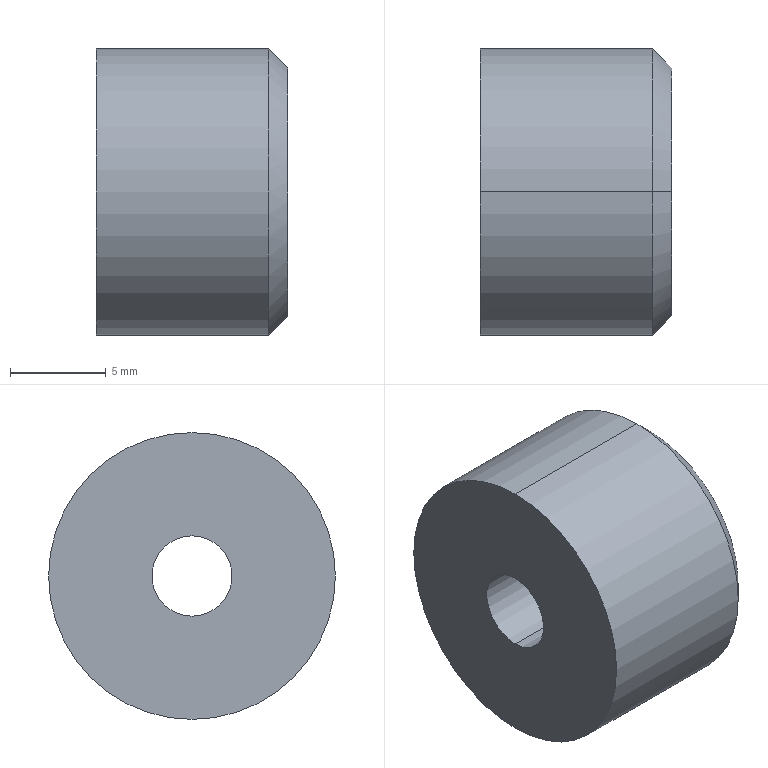Part | SolidWorks | features 3DProfileFeature 1, Chamfer 1, Extrusion 1, HoleWzd 1 | 1 solid | 8 faces | box 10 x 15 x 15 mm | volume 1606 mm3 | cylinder 4 | cone 2 | plane 2 | commonest cylinder face diameters 4.2 x2 15 x2
STEP:
#1=CARTESIAN_POINT('',(2.5,200.,41.6));
#2=VERTEX_POINT('',#1);
#3=CARTESIAN_POINT('',(2.5,200.,37.4));
#4=VERTEX_POINT('',#3);
#5=CARTESIAN_POINT('',(2.5,200.,39.5));
#6=DIRECTION('',(1.,0.,0.));
#7=DIRECTION('',(0.,0.,-1.));
#8=AXIS2_PLACEMENT_3D('',#5,#6,#7);
#9=CIRCLE('',#8,2.1);
#10=EDGE_CURVE('',#2,#4,#9,.T.);
#11=ORIENTED_EDGE('',*,*,#10,.F.);
#12=CARTESIAN_POINT('',(12.5,200.,41.6));
#13=VERTEX_POINT('',#12);
#14=CARTESIAN_POINT('',(12.5,200.,41.6));
#15=DIRECTION('',(1.,0.,0.));
#16=VECTOR('',#15,1000.);
#17=LINE('',#14,#16);
#18=EDGE_CURVE('',#2,#13,#17,.T.);
#19=ORIENTED_EDGE('',*,*,#18,.T.);
#20=CARTESIAN_POINT('',(12.5,200.,37.4));
#21=VERTEX_POINT('',#20);
#22=CARTESIAN_POINT('',(12.5,200.,39.5));
#23=DIRECTION('',(1.,0.,0.));
#24=DIRECTION('',(0.,0.,-1.));
#25=AXIS2_PLACEMENT_3D('',#22,#23,#24);
#26=CIRCLE('',#25,2.1);
#27=EDGE_CURVE('',#13,#21,#26,.T.);
#28=ORIENTED_EDGE('',*,*,#27,.T.);
#29=CARTESIAN_POINT('',(12.5,200.,37.4));
#30=DIRECTION('',(1.,0.,0.));
#31=VECTOR('',#30,1000.);
#32=LINE('',#29,#31);
#33=EDGE_CURVE('',#4,#21,#32,.T.);
#34=ORIENTED_EDGE('',*,*,#33,.F.);
#35=EDGE_LOOP('',(#11,#19,#28,#34));
#36=FACE_OUTER_BOUND('',#35,.T.);
#37=CARTESIAN_POINT('',(12.5,200.,39.5));
#38=DIRECTION('',(1.,0.,0.));
#39=DIRECTION('',(0.,0.,-1.));
#40=AXIS2_PLACEMENT_3D('',#37,#38,#39);
#41=CYLINDRICAL_SURFACE('',#40,2.1);
#42=ADVANCED_FACE('',(#36),#41,.F.);
#43=CARTESIAN_POINT('',(12.5,200.,33.));
#44=VERTEX_POINT('',#43);
#45=CARTESIAN_POINT('',(12.5,200.,46.));
#46=VERTEX_POINT('',#45);
#47=CARTESIAN_POINT('',(12.5,200.,39.5));
#48=DIRECTION('',(1.,0.,0.));
#49=DIRECTION('',(0.,0.,-1.));
#50=AXIS2_PLACEMENT_3D('',#47,#48,#49);
#51=CIRCLE('',#50,6.5);
#52=EDGE_CURVE('',#44,#46,#51,.T.);
#53=ORIENTED_EDGE('',*,*,#52,.F.);
#54=CARTESIAN_POINT('',(11.5,200.,32.));
#55=VERTEX_POINT('',#54);
#56=CARTESIAN_POINT('',(12.5,200.,33.));
#57=DIRECTION('',(-0.7071,0.,-0.7071));
#58=VECTOR('',#57,1000.);
#59=LINE('',#56,#58);
#60=EDGE_CURVE('',#44,#55,#59,.T.);
#61=ORIENTED_EDGE('',*,*,#60,.T.);
#62=CARTESIAN_POINT('',(11.5,200.,47.));
#63=VERTEX_POINT('',#62);
#64=CARTESIAN_POINT('',(11.5,200.,39.5));
#65=DIRECTION('',(-1.,0.,0.));
#66=DIRECTION('',(0.,0.,-1.));
#67=AXIS2_PLACEMENT_3D('',#64,#65,#66);
#68=CIRCLE('',#67,7.5);
#69=EDGE_CURVE('',#63,#55,#68,.T.);
#70=ORIENTED_EDGE('',*,*,#69,.F.);
#71=CARTESIAN_POINT('',(12.5,200.,46.));
#72=DIRECTION('',(-0.7071,0.,0.7071));
#73=VECTOR('',#72,1000.);
#74=LINE('',#71,#73);
#75=EDGE_CURVE('',#46,#63,#74,.T.);
#76=ORIENTED_EDGE('',*,*,#75,.F.);
#77=EDGE_LOOP('',(#53,#61,#70,#76));
#78=FACE_OUTER_BOUND('',#77,.T.);
#79=CARTESIAN_POINT('',(12.5,200.,39.5));
#80=DIRECTION('',(-1.,0.,0.));
#81=DIRECTION('',(0.,0.,1.));
#82=AXIS2_PLACEMENT_3D('',#79,#80,#81);
#83=CONICAL_SURFACE('',#82,6.5,0.7854);
#84=ADVANCED_FACE('',(#78),#83,.T.);
#85=ORIENTED_EDGE('',*,*,#69,.T.);
#86=CARTESIAN_POINT('',(2.5,200.,32.));
#87=VERTEX_POINT('',#86);
#88=CARTESIAN_POINT('',(12.5,200.,32.));
#89=DIRECTION('',(-1.,0.,0.));
#90=VECTOR('',#89,1000.);
#91=LINE('',#88,#90);
#92=EDGE_CURVE('',#55,#87,#91,.T.);
#93=ORIENTED_EDGE('',*,*,#92,.T.);
#94=CARTESIAN_POINT('',(2.5,200.,47.));
#95=VERTEX_POINT('',#94);
#96=CARTESIAN_POINT('',(2.5,200.,39.5));
#97=DIRECTION('',(1.,0.,0.));
#98=DIRECTION('',(0.,0.,-1.));
#99=AXIS2_PLACEMENT_3D('',#96,#97,#98);
#100=CIRCLE('',#99,7.5);
#101=EDGE_CURVE('',#87,#95,#100,.T.);
#102=ORIENTED_EDGE('',*,*,#101,.T.);
#103=CARTESIAN_POINT('',(12.5,200.,47.));
#104=DIRECTION('',(-1.,0.,0.));
#105=VECTOR('',#104,1000.);
#106=LINE('',#103,#105);
#107=EDGE_CURVE('',#63,#95,#106,.T.);
#108=ORIENTED_EDGE('',*,*,#107,.F.);
#109=EDGE_LOOP('',(#85,#93,#102,#108));
#110=FACE_OUTER_BOUND('',#109,.T.);
#111=CARTESIAN_POINT('',(12.5,200.,39.5));
#112=DIRECTION('',(-1.,0.,0.));
#113=DIRECTION('',(0.,0.,1.));
#114=AXIS2_PLACEMENT_3D('',#111,#112,#113);
#115=CYLINDRICAL_SURFACE('',#114,7.5);
#116=ADVANCED_FACE('',(#110),#115,.T.);
#117=ORIENTED_EDGE('',*,*,#92,.F.);
#118=CARTESIAN_POINT('',(11.5,200.,39.5));
#119=DIRECTION('',(-1.,0.,0.));
#120=DIRECTION('',(0.,0.,-1.));
#121=AXIS2_PLACEMENT_3D('',#118,#119,#120);
#122=CIRCLE('',#121,7.5);
#123=EDGE_CURVE('',#55,#63,#122,.T.);
#124=ORIENTED_EDGE('',*,*,#123,.T.);
#125=ORIENTED_EDGE('',*,*,#107,.T.);
#126=CARTESIAN_POINT('',(2.5,200.,39.5));
#127=DIRECTION('',(1.,0.,0.));
#128=DIRECTION('',(0.,0.,-1.));
#129=AXIS2_PLACEMENT_3D('',#126,#127,#128);
#130=CIRCLE('',#129,7.5);
#131=EDGE_CURVE('',#95,#87,#130,.T.);
#132=ORIENTED_EDGE('',*,*,#131,.T.);
#133=EDGE_LOOP('',(#117,#124,#125,#132));
#134=FACE_OUTER_BOUND('',#133,.T.);
#135=CARTESIAN_POINT('',(12.5,200.,39.5));
#136=DIRECTION('',(-1.,0.,0.));
#137=DIRECTION('',(0.,0.,1.));
#138=AXIS2_PLACEMENT_3D('',#135,#136,#137);
#139=CYLINDRICAL_SURFACE('',#138,7.5);
#140=ADVANCED_FACE('',(#134),#139,.T.);
#141=CARTESIAN_POINT('',(12.5,200.,39.5));
#142=DIRECTION('',(1.,0.,0.));
#143=DIRECTION('',(0.,0.,-1.));
#144=AXIS2_PLACEMENT_3D('',#141,#142,#143);
#145=CIRCLE('',#144,2.1);
#146=EDGE_CURVE('',#21,#13,#145,.T.);
#147=ORIENTED_EDGE('',*,*,#146,.F.);
#148=ORIENTED_EDGE('',*,*,#27,.F.);
#149=EDGE_LOOP('',(#147,#148));
#150=FACE_BOUND('',#149,.T.);
#151=CARTESIAN_POINT('',(12.5,200.,39.5));
#152=DIRECTION('',(1.,0.,0.));
#153=DIRECTION('',(0.,0.,-1.));
#154=AXIS2_PLACEMENT_3D('',#151,#152,#153);
#155=CIRCLE('',#154,6.5);
#156=EDGE_CURVE('',#46,#44,#155,.T.);
#157=ORIENTED_EDGE('',*,*,#156,.T.);
#158=ORIENTED_EDGE('',*,*,#52,.T.);
#159=EDGE_LOOP('',(#157,#158));
#160=FACE_OUTER_BOUND('',#159,.T.);
#161=CARTESIAN_POINT('',(12.5,200.,39.5));
#162=DIRECTION('',(1.,0.,0.));
#163=DIRECTION('',(0.,0.,-1.));
#164=AXIS2_PLACEMENT_3D('',#161,#162,#163);
#165=PLANE('',#164);
#166=ADVANCED_FACE('',(#150,#160),#165,.T.);
#167=CARTESIAN_POINT('',(2.5,200.,39.5));
#168=DIRECTION('',(1.,0.,0.));
#169=DIRECTION('',(0.,0.,-1.));
#170=AXIS2_PLACEMENT_3D('',#167,#168,#169);
#171=CIRCLE('',#170,2.1);
#172=EDGE_CURVE('',#4,#2,#171,.T.);
#173=ORIENTED_EDGE('',*,*,#172,.T.);
#174=ORIENTED_EDGE('',*,*,#10,.T.);
#175=EDGE_LOOP('',(#173,#174));
#176=FACE_BOUND('',#175,.T.);
#177=ORIENTED_EDGE('',*,*,#131,.F.);
#178=ORIENTED_EDGE('',*,*,#101,.F.);
#179=EDGE_LOOP('',(#177,#178));
#180=FACE_OUTER_BOUND('',#179,.T.);
#181=CARTESIAN_POINT('',(2.5,200.,39.5));
#182=DIRECTION('',(1.,0.,0.));
#183=DIRECTION('',(0.,0.,-1.));
#184=AXIS2_PLACEMENT_3D('',#181,#182,#183);
#185=PLANE('',#184);
#186=ADVANCED_FACE('',(#176,#180),#185,.F.);
#187=ORIENTED_EDGE('',*,*,#60,.F.);
#188=ORIENTED_EDGE('',*,*,#156,.F.);
#189=ORIENTED_EDGE('',*,*,#75,.T.);
#190=ORIENTED_EDGE('',*,*,#123,.F.);
#191=EDGE_LOOP('',(#187,#188,#189,#190));
#192=FACE_OUTER_BOUND('',#191,.T.);
#193=CARTESIAN_POINT('',(12.5,200.,39.5));
#194=DIRECTION('',(-1.,0.,0.));
#195=DIRECTION('',(0.,0.,1.));
#196=AXIS2_PLACEMENT_3D('',#193,#194,#195);
#197=CONICAL_SURFACE('',#196,6.5,0.7854);
#198=ADVANCED_FACE('',(#192),#197,.T.);
#199=ORIENTED_EDGE('',*,*,#18,.F.);
#200=ORIENTED_EDGE('',*,*,#172,.F.);
#201=ORIENTED_EDGE('',*,*,#33,.T.);
#202=ORIENTED_EDGE('',*,*,#146,.T.);
#203=EDGE_LOOP('',(#199,#200,#201,#202));
#204=FACE_OUTER_BOUND('',#203,.T.);
#205=CARTESIAN_POINT('',(12.5,200.,39.5));
#206=DIRECTION('',(1.,0.,0.));
#207=DIRECTION('',(0.,0.,-1.));
#208=AXIS2_PLACEMENT_3D('',#205,#206,#207);
#209=CYLINDRICAL_SURFACE('',#208,2.1);
#210=ADVANCED_FACE('',(#204),#209,.F.);
#211=CLOSED_SHELL('',(#42,#84,#116,#140,#166,#186,#198,#210));
#212=MANIFOLD_SOLID_BREP('',#211);
#213=CARTESIAN_POINT('',(0.,0.,0.));
#214=DIRECTION('',(0.,0.,1.));
#215=DIRECTION('',(1.,0.,0.));
#216=AXIS2_PLACEMENT_3D('',#213,#214,#215);
#217=(LENGTH_UNIT()NAMED_UNIT(*)SI_UNIT(.MILLI.,.METRE.));
#218=UNCERTAINTY_MEASURE_WITH_UNIT(LENGTH_MEASURE(0.00001),#217,'','');
#219=(NAMED_UNIT(*)PLANE_ANGLE_UNIT()SI_UNIT($,.RADIAN.));
#220=(NAMED_UNIT(*)SI_UNIT($,.STERADIAN.)SOLID_ANGLE_UNIT());
#221=(GEOMETRIC_REPRESENTATION_CONTEXT(3)GLOBAL_UNCERTAINTY_ASSIGNED_CONTEXT((#218))GLOBAL_UNIT_ASSIGNED_CONTEXT((#217,#219,#220))REPRESENTATION_CONTEXT('',''));
#222=ADVANCED_BREP_SHAPE_REPRESENTATION('',(#212,#216),#221);